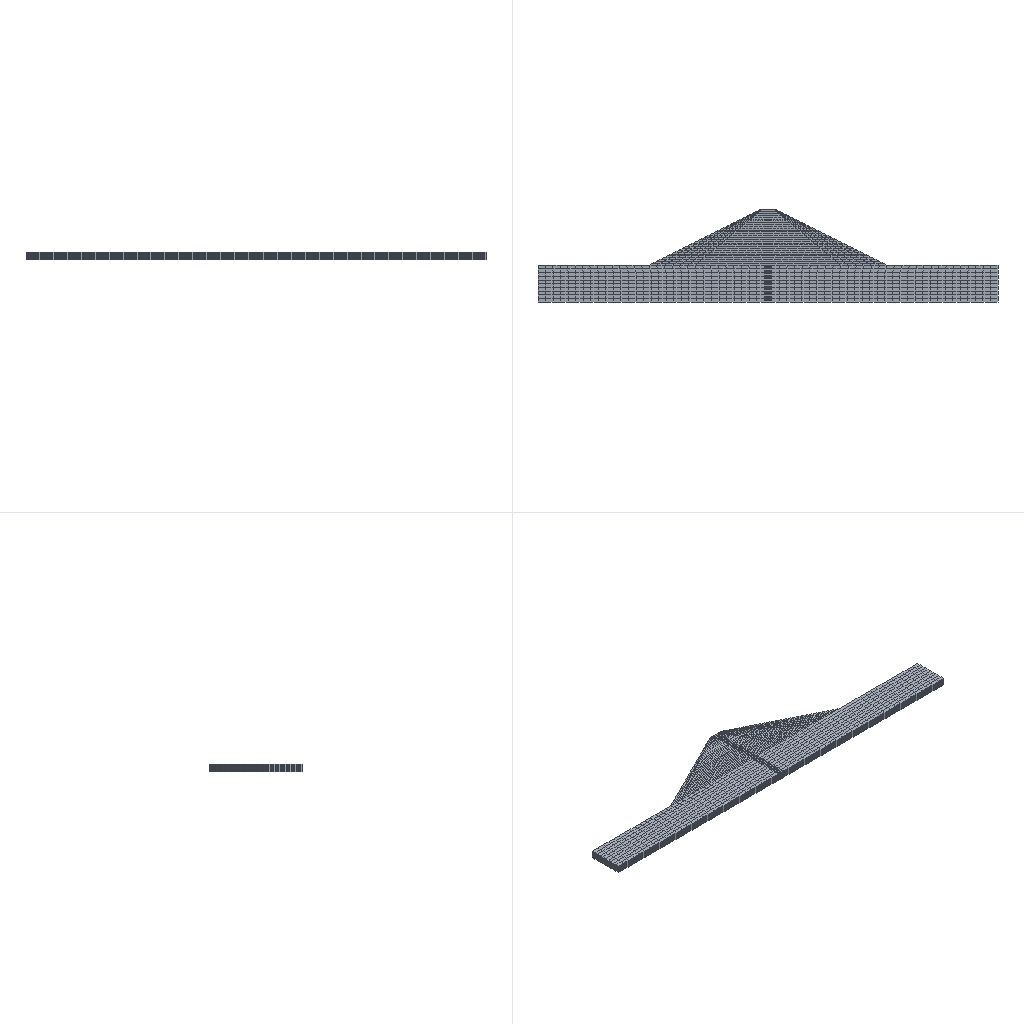Simulation study | abaqus
Set-up summary:
category,name,step,type,value,unit,region
solver,abaqus
solver,version,,,Abaqus/Standard 2020
units,not stated in the deck,,not stated
analysis,deck,,soils,soils
load_step,shenliu,shenliu,soils
load_step,requested,,,1
mesh,nodes,,,23364
mesh,elements,,,19432
element_type,C3D8P,,solid,19432
load,load commands in deck,,count,300
bc,support commands in deck,,count,311
material,BAJI,,in results
material,BATI,,in results
material,QIANG,,in results
check,setup vs results,,match,"per instance, exact: element labels, types and connectivity; labels of the nodes the elements use; coordinates of those nodes at SINGLE_PRECISION in 1 of 2 instance(s)"
Abaqus input file, long lists of numbers shortened:
*Heading
** Job name: Job-4 Model name: 3cm14mML300-OH-shenliu
** Generated by: Abaqus/CAE 2020
*Preprint, echo=NO, model=NO, history=NO, contact=NO
**
** PARTS
**
*Part, name=ba
*End Part
**
*Part, name=qiang
*End Part
**
**
** ASSEMBLY
**
*Assembly, name=Assembly
**
*Instance, name=ba-1, part=ba
*Node
      1,   62.235,         23.5,  0.9
      2,   62.235,         23.5,           0.
** (22570 more lines like these left out)
*Element, type=C3D8P
 1,     1,   169,  2647,   180,   195,  2677, 12325,  2665
 2,   169,   170,  2648,  2647,  2677,  2678, 12326, 12325
** (19078 more lines like these left out)
*Nset, nset=Set-1
     1,     2,     3,     4,     5,     6,     7,     8,     9,    10,    11,    12,    13,    14,    15,    16
    17,    18,    19,    20,    21,    22,    23,    24,    25,    26,    27,    28,    29,    30,    31,    32
** (894 more lines like these left out)
*Elset, elset=Set-1
     1,     2,     3,     4,     5,     6,     7,     8,     9,    10,    11,    12,    13,    14,    15,    16
    17,    18,    19,    20,    21,    22,    23,    24,    25,    26,    27,    28,    29,    30,    31,    32
** (748 more lines like these left out)
*Nset, nset=Set-2
    31,    32,    33,    34,    35,    36,    37,    38,    39,    40,    41,    42,    43,    44,    45,    52
    53,    54,    55,    58,    59,    62,    63,    65,    68,    69,    71,    74,    75,    77,    95,    96
** (543 more lines like these left out)
*Elset, elset=Set-2, generate
  9949,  17028,      1
** Section: bati
*Solid Section, elset=Set-1, material=bati
,
** Section: baji
*Solid Section, elset=Set-2, material=baji
,
*End Instance
**
*Instance, name=qiang-1, part=qiang
      62.235,           8.,           0.
*Node
      1,           0.,         15.5,   1.2
      2, 0.03,         15.5,   1.2
** (790 more lines like these left out)
*Element, type=C3D8P
 1,  84, 111, 110,  33,   1,   2,   3,   4
 2,  83, 112, 109,  34,  84, 111, 110,  33
** (350 more lines like these left out)
*Nset, nset=Set-1, generate
   1,  792,    1
*Elset, elset=Set-1, generate
   1,  352,    1
** Section: qiang
*Solid Section, elset=Set-1, material=qiang
,
*End Instance
**
*Nset, nset=Set-1, instance=ba-1
    31,    32,    33,    34,    35,    36,    37,    38,    39,    40,    41,    42,    43,    44,    45,    52
    53,    54,    55,    58,    59,    62,    63,    65,    68,    69,    71,    74,    75,    77,    95,    96
** (543 more lines like these left out)
*Elset, elset=Set-1, instance=ba-1, generate
  9949,  17028,      1
*Nset, nset=Set-2, instance=ba-1
   131,   132,   133,   134,   135,   136,   138,   139,   143,   144,   145,   146,   147,   148,   154,   155
   156,   158,   162,   163,   165,   166,   167,   168,  1801,  1802,  1803,  1804,  1805,  1806,  1807,  1808
** (14 more lines like these left out)
*Elset, elset=Set-2, instance=ba-1
 10961, 10962, 10963, 10964, 10965, 10966, 10967, 10968, 11085, 11086, 11087, 11088, 11321, 11322, 11323, 11324
 11325, 11326, 11327, 11328, 11525, 11526, 11527, 11528, 11529, 11530, 11531, 11532, 11533, 11534, 11535, 11536
** (11 more lines like these left out)
*Nset, nset=Set-3, instance=ba-1
    97,    98,   101,   102,   104,   106,   108,   109,   112,   115,   116,   117,   121,   122,   124,   125
   151,   152,   153,   154,   155,   156,   157,   158,   159,   160,   161,   162,   163,   164,   165,   167
** (48 more lines like these left out)
*Elset, elset=Set-3, instance=ba-1
  9963,  9964,  9979,  9980,  9995,  9996, 10011, 10012, 10041, 10042, 10043, 10044, 10073, 10074, 10075, 10076
 10105, 10106, 10107, 10108, 10137, 10138, 10139, 10140, 10148, 10156, 10185, 10186, 10187, 10188, 10301, 10302
** (43 more lines like these left out)
*Nset, nset=Set-4, instance=ba-1
     2,     3,     6,     7,    13,    15,    16,    18,    20,    22,    27,    28,    29,    30,    32,    33
    37,    39,    41,    44,    45,    46,    47,    60,    61,    62,    63,    64,    65,    67,    69,    72
** (255 more lines like these left out)
*Nset, nset=Set-4, instance=qiang-1
   9,  10,  11,  12,  17,  18,  19,  20,  21,  22,  23,  24,  26,  27,  31,  32
 145, 146, 147, 148, 149, 150, 151, 152, 153, 154, 155, 156, 157, 158, 159, 160
** (7 more lines like these left out)
*Elset, elset=Set-4, instance=ba-1
     4,     8,    12,    16,    20,    24,    28,    32,    36,    40,    44,    48,    73,    77,    81,    85
    89,    93,    97,   101,   105,   109,   113,   117,   121,   125,   129,   133,   137,   141,   145,   149
** (237 more lines like these left out)
*Elset, elset=Set-4, instance=qiang-1
  30,  33,  36,  39,  42,  45,  48,  51,  54,  57,  60,  63,  66,  69,  72,  75
  78,  81,  84,  87,  90,  93,  96,  99, 102, 105, 108, 114, 117, 120, 121, 122
** (2 more lines like these left out)
*Nset, nset=Set-6, instance=ba-1
     5,     6,    12,    19,    20,    21,    22,    24,    26,    28,    30,    31,    32,    33,    34,    35
    36,    37,    38,    39,    40,    41,    42,    43,    44,    45,    47,    52,    53,    54,    55,    56
** (599 more lines like these left out)
*Nset, nset=Set-6, instance=qiang-1
  13,  14,  15,  16,  17,  18,  19,  20,  21,  22,  23,  24,  25,  26,  27,  28
  29,  30,  31,  32, 205, 206, 207, 208, 213, 214, 215, 216, 217, 218, 219, 220
** (5 more lines like these left out)
*Elset, elset=Set-6, instance=ba-1
    33,    34,    35,    36,    65,    69,   141,   142,   143,   144,   201,   202,   203,   204,   261,   262
   263,   264,   265,   280,   295,   310,   325,   340,   355,   370,   385,   400,   415,   430,   445,   460
** (491 more lines like these left out)
*Elset, elset=Set-6, instance=qiang-1
 111, 118, 119, 120, 121, 122, 123, 126, 129, 132, 135, 138, 141, 142, 143, 144
 145, 146, 147, 148, 149, 150, 151, 152, 153, 154, 155, 156, 157, 158, 159, 160
** (2 more lines like these left out)
*Nset, nset=Set-7, instance=ba-1, generate
     1,  22572,      1
*Nset, nset=Set-7, instance=qiang-1, generate
   1,  792,    1
*Elset, elset=Set-7, instance=ba-1, generate
     1,  19080,      1
*Elset, elset=Set-7, instance=qiang-1, generate
   1,  352,    1
*Nset, nset=Set-8, instance=ba-1
    31,    32,    33,    34,    35,    36,    37,    38,    39,    40,    41,    42,    43,    44,    45,    52
    53,    54,    55,    58,    59,    62,    63,    65,    68,    69,    71,    74,    75,    77,    95,    96
** (543 more lines like these left out)
*Elset, elset=Set-8, instance=ba-1, generate
  9949,  17028,      1
*Nset, nset=Set-9, instance=ba-1
    31,    32,    33,    34,    35,    36,    37,    38,    39,    40,    41,    42,    43,    44,    45,    52
    53,    54,    55,    58,    59,    62,    63,    65,    68,    69,    71,    74,    75,    77,    95,    96
** (543 more lines like these left out)
*Elset, elset=Set-9, instance=ba-1, generate
  9949,  17028,      1
*Nset, nset=Set-10, instance=ba-1
    31,    32,    33,    34,    35,    36,    37,    38,    39,    40,    41,    42,    43,    44,    45,    52
    53,    54,    55,    58,    59,    62,    63,    65,    68,    69,    71,    74,    75,    77,    95,    96
** (543 more lines like these left out)
*Elset, elset=Set-10, instance=ba-1, generate
  9949,  17028,      1
*Nset, nset=Set-12, instance=ba-1
   19,   20,   24,   28,   40,   41,   43,   45,  247,  248,  249,  314,  352,  353,  354,  650
  651,  652,  667,  668,  669,  670,  671,  672,  673,  674,  675,  676,  677,  678,  679,  680
** (18 more lines like these left out)
*Elset, elset=Set-12, instance=ba-1
 1365, 1366, 1367, 1368, 1425, 1426, 1427, 1428, 1485, 1486, 1487, 1488, 1545, 1546, 1547, 1548
 1605, 1606, 1607, 1608, 1665, 1666, 1667, 1668, 1725, 1726, 1727, 1728, 1785, 1786, 1787, 1788
** (15 more lines like these left out)
*Nset, nset=Set-15, instance=ba-1
    31,    32,    33,    34,    35,    36,    37,    38,    39,    40,    41,    42,    43,    44,    45,    52
    53,    54,    55,    58,    59,    62,    63,    65,    68,    69,    71,    74,    75,    77,    95,    96
** (543 more lines like these left out)
*Elset, elset=Set-15, instance=ba-1, generate
  9949,  17028,      1
*Nset, nset=Set-21, instance=ba-1
    31,    32,    33,    34,    35,    36,    37,    38,    39,    40,    41,    42,    43,    44,    45,    52
    53,    54,    55,    58,    59,    62,    63,    65,    68,    69,    71,    74,    75,    77,    95,    96
** (543 more lines like these left out)
*Elset, elset=Set-21, instance=ba-1, generate
  9949,  17028,      1
*Nset, nset=Set-22, instance=ba-1
    31,    32,    33,    34,    35,    36,    37,    38,    39,    40,    41,    42,    43,    44,    45,    52
    53,    54,    55,    58,    59,    62,    63,    65,    68,    69,    71,    74,    75,    77,    95,    96
** (543 more lines like these left out)
*Elset, elset=Set-22, instance=ba-1, generate
  9949,  17028,      1
*Nset, nset=Set-23, instance=ba-1, generate
     1,  22572,      1
*Nset, nset=Set-23, instance=qiang-1, generate
   1,  792,    1
*Elset, elset=Set-23, instance=ba-1, generate
     1,  19080,      1
*Elset, elset=Set-23, instance=qiang-1, generate
   1,  352,    1
*Nset, nset=Set-33, instance=ba-1
    56,    57,    58,    59,    61,    63,    82,    83,    85,    93,    94,   150,  1009,  1038,  1039,  1040
  1041,  1042,  1043,  1044,  1045,  1046,  1047,  1048,  1049,  1050,  1051,  1052,  1053,  1054,  1055,  1056
** (20 more lines like these left out)
*Elset, elset=Set-33, instance=ba-1
  5623,  5638,  5653,  5668,  5683,  5698,  5713,  5728,  5743,  5758,  5773,  5788,  5803,  5818,  5833,  5848
  5863,  5878,  5893,  5908,  5923,  5938,  5953,  5968,  5983,  5998,  6013,  6028,  6043,  6058,  6073,  6088
** (17 more lines like these left out)
*Nset, nset=Set-34, instance=ba-1, generate
     1,  22572,      1
*Nset, nset=Set-34, instance=qiang-1, generate
   1,  792,    1
*Elset, elset=Set-34, instance=ba-1, generate
     1,  19080,      1
*Elset, elset=Set-34, instance=qiang-1, generate
   1,  352,    1
*Nset, nset=Set-35, instance=ba-1
    56,    57,    58,    59,    61,    63,    82,    83,    85,    93,    94,    97,    98,   101,   102,   104
   106,   108,   109,   112,   115,   116,   117,   121,   122,   124,   125,   143,   144,   145,   146,   147
** (86 more lines like these left out)
*Elset, elset=Set-35, instance=ba-1
  5623,  5638,  5653,  5668,  5683,  5698,  5713,  5728,  5743,  5758,  5773,  5788,  5803,  5818,  5833,  5848
  5863,  5878,  5893,  5908,  5923,  5938,  5953,  5968,  5983,  5998,  6013,  6028,  6043,  6058,  6073,  6088
** (76 more lines like these left out)
*Nset, nset=Set-36, instance=ba-1, generate
     1,  22572,      1
*Nset, nset=Set-36, instance=qiang-1, generate
   1,  792,    1
*Elset, elset=Set-36, instance=ba-1, generate
     1,  19080,      1
*Elset, elset=Set-36, instance=qiang-1, generate
   1,  352,    1
*Nset, nset=Set-39, instance=ba-1
   151,   152,   153,   154,   155,   156,   157,   158,   159,   160,   161,   162,   163,   164,   165,   167
  2188,  2189,  2190,  2198,  2199,  2200,  2201,  2202,  2203,  2204,  2205,  2206,  2207,  2208,  2209,  2210
** (37 more lines like these left out)
*Elset, elset=Set-39, instance=ba-1
 11877, 11878, 11879, 11880, 11881, 11882, 11883, 11884, 11885, 11886, 11887, 11888, 11889, 11890, 11891, 11892
 11893, 11894, 11895, 11896, 11897, 11898, 11899, 11900, 11901, 11902, 11903, 11904, 11905, 11906, 11907, 11908
** (28 more lines like these left out)
*Nset, nset=Set-41, instance=ba-1
   130,   132,   137,   138,   140,   147,   149,   153,   154,   157,   158,   159,   164,   165,   166,   167
  1866,  1867,  1868,  1869,  1870,  1871,  1872,  1873,  1874,  1875,  1876,  1877,  1878,  1879,  1880,  1881
** (68 more lines like these left out)
*Elset, elset=Set-41, instance=ba-1
 11880, 11884, 11888, 11892, 11896, 11900, 11904, 11908, 11912, 11916, 11920, 11924, 11928, 11932, 11936, 11940
 11944, 11948, 11952, 11956, 11960, 11964, 11968, 11972, 11976, 11980, 11984, 11988, 11992, 11996, 12000, 12004
** (58 more lines like these left out)
*Nset, nset=Set-44, instance=ba-1
    97,    98,   101,   102,   104,   106,   108,   109,   112,   115,   116,   117,   121,   122,   124,   125
   151,   152,   153,   154,   155,   156,   157,   158,   159,   160,   161,   162,   163,   164,   165,   167
** (48 more lines like these left out)
*Elset, elset=Set-44, instance=ba-1
  9963,  9964,  9979,  9980,  9995,  9996, 10011, 10012, 10041, 10042, 10043, 10044, 10073, 10074, 10075, 10076
 10105, 10106, 10107, 10108, 10137, 10138, 10139, 10140, 10148, 10156, 10185, 10186, 10187, 10188, 10301, 10302
** (43 more lines like these left out)
*Nset, nset=Set-45, instance=ba-1
     2,     3,    13,    15,    20,    27,    28,    32,    33,    37,    39,    41,    44,    45,    46,    60
    61,    62,    63,    64,    65,    67,    69,    72,    73,    74,    75,    76,    77,    93,   103,   104
** (239 more lines like these left out)
*Nset, nset=Set-45, instance=qiang-1
   9,  10,  11,  12,  19,  20,  23,  24,  26,  27, 145, 146, 147, 148, 149, 150
 151, 152, 153, 154, 155, 156, 157, 158, 159, 160, 161, 162, 163, 164, 165, 166
** (6 more lines like these left out)
*Elset, elset=Set-45, instance=ba-1
   556,   560,   564,   568,   572,   576,   580,   584,   588,   592,   596,   600,   604,   608,   612,   616
   620,   624,   628,   632,   636,   640,   644,   648,   652,   656,   660,   664,   668,   672,   676,   680
** (221 more lines like these left out)
*Elset, elset=Set-45, instance=qiang-1
  30,  33,  36,  39,  42,  45,  48,  51,  54,  57,  60,  63,  66,  69,  72,  75
  78,  81,  84,  87,  90,  93,  96,  99, 102, 105, 108, 142, 143, 144, 145, 146
** (2 more lines like these left out)
*Elset, elset=_Surf-26_S2, internal, instance=ba-1
  551,  552, 9353, 9354
*Surface, type=ELEMENT, name=Surf-26
_Surf-26_S2, S2
*Elset, elset=_Surf-27_S5, internal, instance=ba-1
 6489, 6490, 6491, 6492, 6549, 6550, 6551, 6552, 6609, 6610, 6611, 6612, 6669, 6670, 6671, 6672
 6729, 6730, 6731, 6732, 6789, 6790, 6791, 6792, 6849, 6850, 6851, 6852, 6909, 6910, 6911, 6912
** (5 more lines like these left out)
*Elset, elset=_Surf-27_S6, internal, instance=ba-1, generate
 5623,  6418,    15
*Elset, elset=_Surf-27_S2, internal, instance=ba-1, generate
 17029,  17136,      1
*Surface, type=ELEMENT, name=Surf-27
_Surf-27_S5, S5
_Surf-27_S6, S6
_Surf-27_S2, S2
*Elset, elset=_Surf-28_S5, internal, instance=ba-1
 6489, 6490, 6491, 6492, 6549, 6550, 6551, 6552, 6609, 6610, 6611, 6612, 6669, 6670, 6671, 6672
 6729, 6730, 6731, 6732, 6789, 6790, 6791, 6792, 6849, 6850, 6851, 6852, 6909, 6910, 6911, 6912
** (5 more lines like these left out)
*Elset, elset=_Surf-28_S6, internal, instance=ba-1, generate
 5623,  6418,    15
*Elset, elset=_Surf-28_S2, internal, instance=ba-1, generate
 17029,  17136,      1
*Surface, type=ELEMENT, name=Surf-28
_Surf-28_S5, S5
_Surf-28_S6, S6
_Surf-28_S2, S2
*Elset, elset=_ba-xia_S6, internal, instance=ba-1
 10141, 10149, 10317, 10325, 10333, 10341
*Elset, elset=_ba-xia_S3, internal, instance=ba-1, generate
 10157,  10160,      1
*Surface, type=ELEMENT, name=ba-xia
_ba-xia_S6, S6
_ba-xia_S3, S3
*Elset, elset=_ba-you_S5, internal, instance=ba-1
  8821,  8822,  8823,  8824,  8837,  8838,  8839,  8840,  8853,  8854,  8855,  8856,  8869,  8870,  8871,  8872
  8885,  8886,  8887,  8888,  8901,  8902,  8903,  8904,  8917,  8918,  8919,  8920,  8933,  8934,  8935,  8936
** (7 more lines like these left out)
*Elset, elset=_ba-you_S6, internal, instance=ba-1
 8161, 8165, 8169, 8173, 8177, 8181, 8185, 8189, 8193, 8197, 8201, 8205, 8209, 8213, 8217, 8221
 8225, 8229, 8233, 8237, 8241, 8245, 8249, 8253, 8257, 8261, 8265, 8269, 8273, 8277, 8281, 8285
** (10 more lines like these left out)
*Elset, elset=_ba-you_S3, internal, instance=ba-1
 11773, 11774, 11781, 11782
*Surface, type=ELEMENT, name=ba-you
_ba-you_S5, S5
_ba-you_S6, S6
_ba-you_S3, S3
*Elset, elset=_ba-zuo_S3, internal, instance=ba-1
     1,     2,     3,     4,    17,    18,    19,    20,    33,    34,    35,    36,   553,   554,   555,   556
   569,   570,   571,   572,   585,   586,   587,   588,   601,   602,   603,   604,   617,   618,   619,   620
** (6 more lines like these left out)
*Elset, elset=_ba-zuo_S6, internal, instance=ba-1
    49,    53,    57,    61,    65,    69,   985,   989,   993,   997,  1001,  1005,  1009,  1013,  1017,  1021
  1025,  1029,  1033,  1037,  1041,  1045,  1049,  1053,  1057,  1061,  1065,  1069,  1073,  1077,  1081,  1085
** (2 more lines like these left out)
*Elset, elset=_ba-zuo_S1, internal, instance=ba-1
  5557,  5558,  5559,  5560,  5561,  5562,  5563,  5564,  5565,  5566,  5567,  5568, 18973, 18974, 18975, 18976
 18977, 18978, 18979, 18980, 18981, 18982, 18983, 18984, 18985, 18986, 18987, 18988, 18989, 18990, 18991, 18992
** (6 more lines like these left out)
*Elset, elset=_ba-zuo_S5, internal, instance=ba-1
 10701, 10702, 10703, 10704, 10717, 10718, 10719, 10720
*Surface, type=ELEMENT, name=ba-zuo
_ba-zuo_S3, S3
_ba-zuo_S6, S6
_ba-zuo_S1, S1
_ba-zuo_S5, S5
*Elset, elset=_baxia_S2, internal, instance=ba-1
  9769,  9770,  9771,  9772,  9773,  9774,  9775,  9776,  9777,  9778,  9779,  9780, 17029, 17030, 17031, 17032
 17033, 17034, 17035, 17036, 17037, 17038, 17039, 17040, 17041, 17042, 17043, 17044, 17045, 17046, 17047, 17048
** (6 more lines like these left out)
*Elset, elset=_baxia_S6, internal, instance=ba-1
 5623, 5638, 5653, 5668, 5683, 5698, 5713, 5728, 5743, 5758, 5773, 5788, 5803, 5818, 5833, 5848
 5863, 5878, 5893, 5908, 5923, 5938, 5953, 5968, 5983, 5998, 6013, 6028, 6043, 6058, 6073, 6088
** (2 more lines like these left out)
*Elset, elset=_baxia_S5, internal, instance=ba-1
 6489, 6490, 6491, 6492, 6549, 6550, 6551, 6552, 6609, 6610, 6611, 6612, 6669, 6670, 6671, 6672
 6729, 6730, 6731, 6732, 6789, 6790, 6791, 6792, 6849, 6850, 6851, 6852, 6909, 6910, 6911, 6912
** (6 more lines like these left out)
*Surface, type=ELEMENT, name=baxia
_baxia_S2, S2
_baxia_S6, S6
_baxia_S5, S5
*Elset, elset=_fdown_S2, internal, instance=ba-1
  9769,  9770,  9771,  9772,  9773,  9774,  9775,  9776,  9777,  9778,  9779,  9780, 17029, 17030, 17031, 17032
 17033, 17034, 17035, 17036, 17037, 17038, 17039, 17040, 17041, 17042, 17043, 17044, 17045, 17046, 17047, 17048
** (6 more lines like these left out)
*Elset, elset=_fdown_S6, internal, instance=ba-1
 5623, 5638, 5653, 5668, 5683, 5698, 5713, 5728, 5743, 5758, 5773, 5788, 5803, 5818, 5833, 5848
 5863, 5878, 5893, 5908, 5923, 5938, 5953, 5968, 5983, 5998, 6013, 6028, 6043, 6058, 6073, 6088
** (2 more lines like these left out)
*Elset, elset=_fdown_S5, internal, instance=ba-1
 6489, 6490, 6491, 6492, 6549, 6550, 6551, 6552, 6609, 6610, 6611, 6612, 6669, 6670, 6671, 6672
 6729, 6730, 6731, 6732, 6789, 6790, 6791, 6792, 6849, 6850, 6851, 6852, 6909, 6910, 6911, 6912
** (6 more lines like these left out)
*Surface, type=ELEMENT, name=fdown
_fdown_S2, S2
_fdown_S6, S6
_fdown_S5, S5
*Elset, elset=_m_Surf-14_S3, internal, instance=ba-1
     1,     2,     3,     4,    17,    18,    19,    20,    33,    34,    35,    36,   553,   554,   555,   556
   569,   570,   571,   572,   585,   586,   587,   588,   601,   602,   603,   604,   617,   618,   619,   620
** (6 more lines like these left out)
*Elset, elset=_m_Surf-14_S6, internal, instance=ba-1
    49,    53,    57,    61,    65,    69,   985,   989,   993,   997,  1001,  1005,  1009,  1013,  1017,  1021
  1025,  1029,  1033,  1037,  1041,  1045,  1049,  1053,  1057,  1061,  1065,  1069,  1073,  1077,  1081,  1085
** (2 more lines like these left out)
*Elset, elset=_m_Surf-14_S1, internal, instance=ba-1
  5557,  5558,  5559,  5560,  5561,  5562,  5563,  5564,  5565,  5566,  5567,  5568, 18973, 18974, 18975, 18976
 18977, 18978, 18979, 18980, 18981, 18982, 18983, 18984, 18985, 18986, 18987, 18988, 18989, 18990, 18991, 18992
** (6 more lines like these left out)
*Elset, elset=_m_Surf-14_S5, internal, instance=ba-1
 10701, 10702, 10703, 10704, 10717, 10718, 10719, 10720
*Surface, type=ELEMENT, name=m_Surf-14
_m_Surf-14_S3, S3
_m_Surf-14_S6, S6
_m_Surf-14_S1, S1
_m_Surf-14_S5, S5
*Elset, elset=_m_Surf-16_S5, internal, instance=ba-1
  8821,  8822,  8823,  8824,  8837,  8838,  8839,  8840,  8853,  8854,  8855,  8856,  8869,  8870,  8871,  8872
  8885,  8886,  8887,  8888,  8901,  8902,  8903,  8904,  8917,  8918,  8919,  8920,  8933,  8934,  8935,  8936
** (7 more lines like these left out)
*Elset, elset=_m_Surf-16_S6, internal, instance=ba-1
 8161, 8165, 8169, 8173, 8177, 8181, 8185, 8189, 8193, 8197, 8201, 8205, 8209, 8213, 8217, 8221
 8225, 8229, 8233, 8237, 8241, 8245, 8249, 8253, 8257, 8261, 8265, 8269, 8273, 8277, 8281, 8285
** (10 more lines like these left out)
*Elset, elset=_m_Surf-16_S3, internal, instance=ba-1
 11773, 11774, 11781, 11782
*Surface, type=ELEMENT, name=m_Surf-16
_m_Surf-16_S5, S5
_m_Surf-16_S6, S6
_m_Surf-16_S3, S3
*Elset, elset=_m_Surf-18_S6, internal, instance=ba-1
 10141, 10149, 10317, 10325, 10333, 10341
*Elset, elset=_m_Surf-18_S3, internal, instance=ba-1, generate
 10157,  10160,      1
*Surface, type=ELEMENT, name=m_Surf-18
_m_Surf-18_S6, S6
_m_Surf-18_S3, S3
*Elset, elset=_qiang-xia_S6, internal, instance=qiang-1, generate
 331,  351,    2
*Surface, type=ELEMENT, name=qiang-xia
_qiang-xia_S6, S6
*Elset, elset=_qiang-you_S5, internal, instance=qiang-1
  28,  29,  30,  31,  32,  33,  34,  35,  36,  37,  38,  39,  40,  41,  42,  43
  44,  45,  46,  47,  48,  49,  50,  51,  52,  53,  54,  55,  56,  57,  58,  59
** (4 more lines like these left out)
*Elset, elset=_qiang-you_S4, internal, instance=qiang-1
   1,   2,   3,   4,   5,   6,   7,   8,   9,  10,  11,  12,  13,  14,  15,  16
  17,  18,  19,  20,  21,  22,  23,  24,  25,  26,  27, 109, 110, 111, 142, 143
** (12 more lines like these left out)
*Elset, elset=_qiang-you_S6, internal, instance=qiang-1, generate
 121,  141,    1
*Elset, elset=_qiang-you_S3, internal, instance=qiang-1, generate
 345,  352,    1
*Elset, elset=_qiang-you_S1, internal, instance=qiang-1, generate
 331,  344,    1
*Surface, type=ELEMENT, name=qiang-you
_qiang-you_S5, S5
_qiang-you_S4, S4
_qiang-you_S6, S6
_qiang-you_S3, S3
_qiang-you_S1, S1
*Elset, elset=_qiang-zuo_S3, internal, instance=qiang-1
  28,  29,  30,  31,  32,  33,  34,  35,  36,  37,  38,  39,  40,  41,  42,  43
  44,  45,  46,  47,  48,  49,  50,  51,  52,  53,  54,  55,  56,  57,  58,  59
** (4 more lines like these left out)
*Elset, elset=_qiang-zuo_S4, internal, instance=qiang-1, generate
 121,  141,    1
*Elset, elset=_qiang-zuo_S6, internal, instance=qiang-1
   1,   2,   3,   4,   5,   6,   7,   8,   9,  10,  11,  12,  13,  14,  15,  16
  17,  18,  19,  20,  21,  22,  23,  24,  25,  26,  27, 109, 110, 111, 142, 143
** (12 more lines like these left out)
*Elset, elset=_qiang-zuo_S2, internal, instance=qiang-1, generate
 331,  344,    1
*Elset, elset=_qiang-zuo_S5, internal, instance=qiang-1, generate
 345,  352,    1
*Surface, type=ELEMENT, name=qiang-zuo
_qiang-zuo_S3, S3
_qiang-zuo_S4, S4
_qiang-zuo_S6, S6
_qiang-zuo_S2, S2
_qiang-zuo_S5, S5
*Elset, elset=_qiangdi_S2, internal, instance=qiang-1
 111, 118, 119, 120
*Elset, elset=_qiangdi_S5, internal, instance=qiang-1, generate
 123,  141,    3
*Surface, type=ELEMENT, name=qiangdi
_qiangdi_S2, S2
_qiangdi_S5, S5
*Elset, elset=_s_Surf-14_S3, internal, instance=qiang-1
  28,  29,  30,  31,  32,  33,  34,  35,  36,  37,  38,  39,  40,  41,  42,  43
  44,  45,  46,  47,  48,  49,  50,  51,  52,  53,  54,  55,  56,  57,  58,  59
** (4 more lines like these left out)
*Elset, elset=_s_Surf-14_S4, internal, instance=qiang-1, generate
 121,  141,    1
*Elset, elset=_s_Surf-14_S6, internal, instance=qiang-1
   1,   2,   3,   4,   5,   6,   7,   8,   9,  10,  11,  12,  13,  14,  15,  16
  17,  18,  19,  20,  21,  22,  23,  24,  25,  26,  27, 109, 110, 111, 142, 143
** (12 more lines like these left out)
*Elset, elset=_s_Surf-14_S2, internal, instance=qiang-1, generate
 331,  344,    1
*Elset, elset=_s_Surf-14_S5, internal, instance=qiang-1, generate
 345,  352,    1
*Surface, type=ELEMENT, name=s_Surf-14
_s_Surf-14_S3, S3
_s_Surf-14_S4, S4
_s_Surf-14_S6, S6
_s_Surf-14_S2, S2
_s_Surf-14_S5, S5
*Elset, elset=_s_Surf-16_S5, internal, instance=qiang-1
  28,  29,  30,  31,  32,  33,  34,  35,  36,  37,  38,  39,  40,  41,  42,  43
  44,  45,  46,  47,  48,  49,  50,  51,  52,  53,  54,  55,  56,  57,  58,  59
** (4 more lines like these left out)
*Elset, elset=_s_Surf-16_S4, internal, instance=qiang-1
   1,   2,   3,   4,   5,   6,   7,   8,   9,  10,  11,  12,  13,  14,  15,  16
  17,  18,  19,  20,  21,  22,  23,  24,  25,  26,  27, 109, 110, 111, 142, 143
** (12 more lines like these left out)
*Elset, elset=_s_Surf-16_S6, internal, instance=qiang-1, generate
 121,  141,    1
*Elset, elset=_s_Surf-16_S3, internal, instance=qiang-1, generate
 345,  352,    1
*Elset, elset=_s_Surf-16_S1, internal, instance=qiang-1, generate
 331,  344,    1
*Surface, type=ELEMENT, name=s_Surf-16
_s_Surf-16_S5, S5
_s_Surf-16_S4, S4
_s_Surf-16_S6, S6
_s_Surf-16_S3, S3
_s_Surf-16_S1, S1
*Elset, elset=_s_Surf-18_S6, internal, instance=qiang-1, generate
 331,  351,    2
*Surface, type=ELEMENT, name=s_Surf-18
_s_Surf-18_S6, S6
*Nset, nset=Set-12_PP_, internal, instance=ba-1
   19,   20,   24,   28,   40,   41,   43,   45,  247,  248,  249,  314,  352,  353,  354,  650
  651,  652,  667,  668,  669,  670,  671,  672,  673,  674,  675,  676,  677,  678,  679,  680
** (18 more lines like these left out)
*End Assembly
**
** MATERIALS
**
*Material, name=baji
*Density
2200.,
*Elastic
 2e+08, 0.29
*Gap Flow
 0.0001,
*Permeability, specific=1000.
 1e-07, 1.5
*Material, name=bati
*Density
1930.,
*Elastic
 1e+08, 0.29
*Gap Flow
 0.0001,
*Permeability, specific=1000.
 5e-07, 1.5
*Permeability, Type=SATURATION
     1e-05, 0.02154
    0.0001, 0.04642
     0.001,       0.1
 0.07244,  0.4169
  0.9703,      0.99
        1.,        1.
*Sorption
-200000., 0.02154
-150000., 0.04642
-100000.,       0.1
 -50000.,  0.4169
 -20000.,      0.99
      0.,        1.
*Material, name=qiang
*Density
300.,
*Elastic
 1.00176e+08, 0.272
*Gap Flow
 0.0001,
*Permeability, specific=1000.
 1e-10, 1.5
**
** INTERACTION PROPERTIES
**
*Surface Interaction, name=IntProp-1
1.,
*Friction, slip tolerance=0.005
 0.1,
*Surface Behavior, penalty
**
** BOUNDARY CONDITIONS
**
** Name: x Type: Displacement/Rotation
*Boundary
Set-2, 1, 1
** PREDEFINED FIELDS
**
** Name: Predefined Field-1   Type: Saturation
*Initial Conditions, type=SATURATION
Set-7, 1.
** Name: Predefined Field-2   Type: Void ratio
*Initial Conditions, TYPE=RATIO
Set-7, 0.8
**
** INTERACTIONS
**
** Interaction: Int-4
*Contact
*Contact Inclusions, ALL EXTERIOR
*Contact Property Assignment
 ,  , IntProp-1
** ----------------------------------------------------------------
**
** STEP: shenliu
**
*Step, name=shenliu, nlgeom=NO, inc=1000
*Soils, utol=1.0, creep=none, stabilize=0.0002, allsdtol=0, continue=NO
0.001, 1., 1e-10, 1.,
*sflow
fdown,qd,0.1
**
** BOUNDARY CONDITIONS
**
** Name: BC-4 Type: 对称/反对称/完全固定
*Boundary
Set-44, ENCASTRE
** Name: BC-5 Type: 位移/转角
*Boundary
Set-45, 3, 3
** Name: shenliu Type: Pore pressure Using Analytical Field: shenliu135
*Boundary
ba-1.19, 8, 8, 0.
ba-1.20, 8, 8, 0.
ba-1.24, 8, 8, 0.
ba-1.28, 8, 8, 0.
ba-1.40, 8, 8, 135000.
ba-1.41, 8, 8, 135000.
ba-1.43, 8, 8, 135000.
ba-1.45, 8, 8, 135000.
ba-1.247, 8, 8, 0.
ba-1.248, 8, 8, 0.
ba-1.249, 8, 8, 0.
ba-1.314, 8, 8, 0.
ba-1.352, 8, 8, 0.
ba-1.353, 8, 8, 0.
ba-1.354, 8, 8, 0.
ba-1.650, 8, 8, 135000.
ba-1.651, 8, 8, 135000.
ba-1.652, 8, 8, 135000.
ba-1.667, 8, 8, 5000.
ba-1.668, 8, 8, 10000.
ba-1.669, 8, 8, 15000.
ba-1.670, 8, 8, 20000.
ba-1.671, 8, 8, 25000.
ba-1.672, 8, 8, 30000.
ba-1.673, 8, 8, 35000.
ba-1.674, 8, 8, 40000.
ba-1.675, 8, 8, 45000.
ba-1.676, 8, 8, 50000.
ba-1.677, 8, 8, 55000.
ba-1.678, 8, 8, 60000.
ba-1.679, 8, 8, 65000.
ba-1.680, 8, 8, 70000.
ba-1.681, 8, 8, 75000.
ba-1.682, 8, 8, 80000.
ba-1.683, 8, 8, 85000.
ba-1.684, 8, 8, 90000.
ba-1.685, 8, 8, 95000.
ba-1.686, 8, 8, 100000.
ba-1.687, 8, 8, 105000.
ba-1.688, 8, 8, 110000.
** (268 more lines like these left out)
**
** LOADS
**
** Name: Load-3   Type: Pressure
*Dsload
Surf-26, P, 500000.
** Name: Load-4   Type: Gravity
*Dload
, GRAV, 9.8, 0., -1., 0.
**
** CONTROLS
**
*Controls, reset
*Controls, parameters=time incrementation
, , , , , , , 20, , ,
**
** OUTPUT REQUESTS
**
*Restart, write, frequency=0
**
** FIELD OUTPUT: F-Output-2
**
*Output, field
*Node Output
POR, RF, U
*Element Output, directions=YES
E, MISES, PEMAG, S, SAT, VOIDR
*Contact Output
CSTRESS,
**
** HISTORY OUTPUT: H-Output-3
**
*Output, history
*Energy Output
ALLAE,
*End Step
Results summary:
result,step,,partial,increments=5 time=0.009125/1.0
result,analysis,,,soils
result,last_loadstep,,,1
result,primary field,,,"U, POR"
result,reaction total,,FX,1.6e-05,model units
result,reaction total,,FY,717324.967,model units
result,reaction total,,FZ,-0.001852,model units